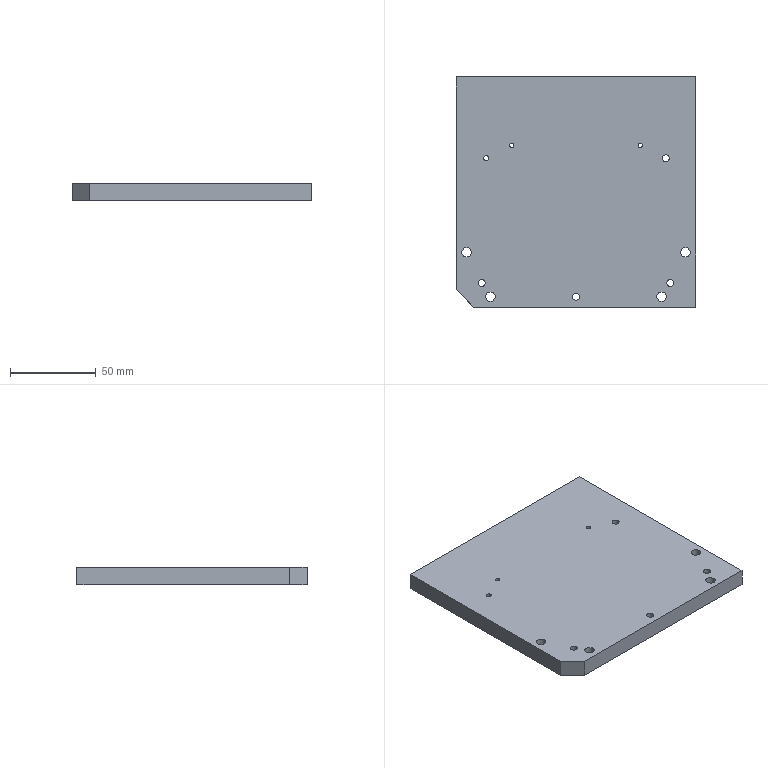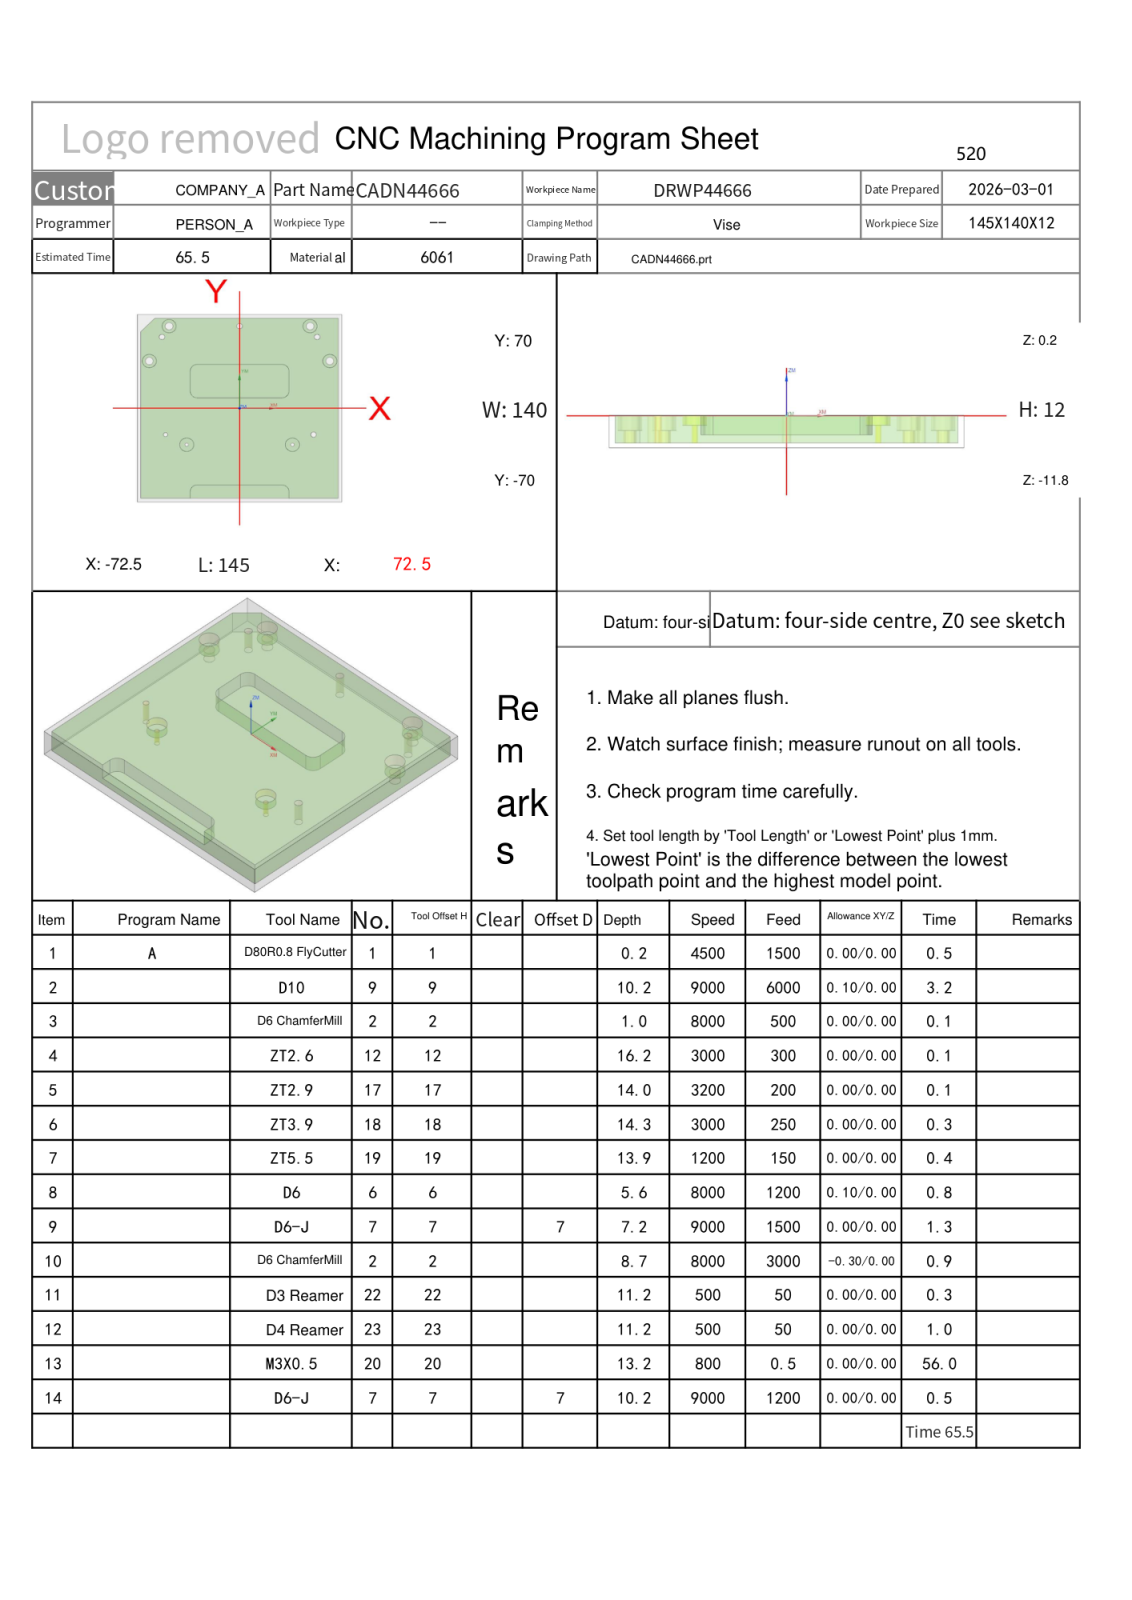NC program | NX | posted by the shop | part box 140 x 134.5 x 10 mm
Whole program:
%
O0001
(Machine time: 120.02 MIN)
(===Total Tool:12===)
(T1=D80R0.8 FlyCutter D=80.  R=0.8  D-  H01 Z=0.    )
(T9=D10     D=10.  R=0.   D9  H09 Z=-10.  )
(T2=D6 ChamferMill   D=6.   R=0.   D-  H02 Z=-8.5  )
(T12=ZT2.6  D=2.6  DR_a=118 D-  H12 Z=-16.  )
(T17=ZT2.9  D=2.9  DR_a=120 D-  H17 Z=-13.84)
(T18=ZT3.9  D=3.9  DR_a=120 D-  H18 Z=-14.13)
(T19=ZT5.5  D=5.5  DR_a=118 D-  H19 Z=-13.65)
(T6=D6      D=6.   R=0.   D-  H06 Z=-5.4  )
(T7=D6-J    D=6.   R=0.   D7  H07 Z=-10.  )
(T22=D3 Reamer   D=3.   DR_a=180 D-  H22 Z=-11.  )
(T23=D4 Reamer   D=4.   DR_a=180 D-  H23 Z=-11.  )
(T20=M3X0.5 D=2.5  DR_a=180 D-  H20 Z=-13.  )
G80 G90 G17 G49 G40
G91 G28 Z0
M01
N1 T01 M06
(D80R0.8 FlyCutter  D=80. R=0.8 H=01 ce=0.00 di=0.00)
G00 G90 G54 X115. Y-53.625 M03 S4500
G43 H01 Z50.
M08
Z2.
G01 Z0.0 F1500.
X110.
X-110.
Y0.0
X110.
Y53.625
X-110.
X-115.
Z2.
G00 Z50.
G91 G28 Z0.0
M05
M09
G91 G28 Z0.0
M01
N2 T09 M06
(D10  D=10. R=0. H=09 ce=0.10 di=0.00)
G00 G90 G54 X0.0 Y-72.35 M03 S8000
G43 H09 Z50.
M08
Z.5
G01 X-70. Z.409 F6000.
G02 X-75.1 Y-67.25 Z.398 I0.0 J5.1
G01 Y57.25 Z.236
G02 X-73.606 Y60.856 Z.231 I5.1 J0.0
G01 X-63.606 Y70.856 Z.212
G02 X-60. Y72.35 Z.207 I3.606 J-3.606
G01 X70. Z.038
G02 X75.1 Y67.25 Z.027 I0.0 J-5.1
G01 Y-67.25 Z-.148
G02 X70. Y-72.35 Z-.159 I-5.1 J0.0
G01 X-70. Z-.341
G02 X-75.1 Y-67.25 Z-.352 I0.0 J5.1
G01 Y57.25 Z-.514
G02 X-73.606 Y60.856 Z-.519 I5.1 J0.0
G01 X-63.606 Y70.856 Z-.538
G02 X-60. Y72.35 Z-.543 I3.606 J-3.606
G01 X70. Z-.712
G02 X75.1 Y67.25 Z-.723 I0.0 J-5.1
G01 Y-67.25 Z-.898
G02 X70. Y-72.35 Z-.909 I-5.1 J0.0
G01 X-70. Z-1.091
G02 X-75.1 Y-67.25 Z-1.102 I0.0 J5.1
G01 Y57.25 Z-1.264
G02 X-73.606 Y60.856 Z-1.269 I5.1 J0.0
G01 X-63.606 Y70.856 Z-1.288
G02 X-60. Y72.35 Z-1.293 I3.606 J-3.606
G01 X70. Z-1.462
G02 X75.1 Y67.25 Z-1.473 I0.0 J-5.1
G01 Y-67.25 Z-1.648
G02 X70. Y-72.35 Z-1.659 I-5.1 J0.0
G01 X-70. Z-1.841
G02 X-75.1 Y-67.25 Z-1.852 I0.0 J5.1
G01 Y57.25 Z-2.014
G02 X-73.606 Y60.856 Z-2.019 I5.1 J0.0
G01 X-63.606 Y70.856 Z-2.038
G02 X-60. Y72.35 Z-2.043 I3.606 J-3.606
G01 X70. Z-2.212
G02 X75.1 Y67.25 Z-2.223 I0.0 J-5.1
G01 Y-67.25 Z-2.398
G02 X70. Y-72.35 Z-2.409 I-5.1 J0.0
G01 X-70. Z-2.591
G02 X-75.1 Y-67.25 Z-2.602 I0.0 J5.1
G01 Y57.25 Z-2.764
G02 X-73.606 Y60.856 Z-2.769 I5.1 J0.0
G01 X-63.606 Y70.856 Z-2.788
G02 X-60. Y72.35 Z-2.793 I3.606 J-3.606
G01 X70. Z-2.962
G02 X75.1 Y67.25 Z-2.973 I0.0 J-5.1
G01 Y-67.25 Z-3.148
G02 X70. Y-72.35 Z-3.159 I-5.1 J0.0
G01 X-70. Z-3.341
G02 X-75.1 Y-67.25 Z-3.352 I0.0 J5.1
G01 Y57.25 Z-3.514
G02 X-73.606 Y60.856 Z-3.519 I5.1 J0.0
G01 X-63.606 Y70.856 Z-3.538
G02 X-60. Y72.35 Z-3.543 I3.606 J-3.606
G01 X70. Z-3.712
G02 X75.1 Y67.25 Z-3.723 I0.0 J-5.1
G01 Y-67.25 Z-3.898
G02 X70. Y-72.35 Z-3.909 I-5.1 J0.0
G01 X-70. Z-4.091
G02 X-75.1 Y-67.25 Z-4.102 I0.0 J5.1
G01 Y57.25 Z-4.264
G02 X-73.606 Y60.856 Z-4.269 I5.1 J0.0
G01 X-63.606 Y70.856 Z-4.288
G02 X-60. Y72.35 Z-4.293 I3.606 J-3.606
G01 X70. Z-4.462
G02 X75.1 Y67.25 Z-4.473 I0.0 J-5.1
G01 Y-67.25 Z-4.648
G02 X70. Y-72.35 Z-4.659 I-5.1 J0.0
G01 X-70. Z-4.841
G02 X-75.1 Y-67.25 Z-4.852 I0.0 J5.1
G01 Y57.25 Z-5.014
G02 X-73.606 Y60.856 Z-5.019 I5.1 J0.0
G01 X-63.606 Y70.856 Z-5.038
G02 X-60. Y72.35 Z-5.043 I3.606 J-3.606
G01 X70. Z-5.212
G02 X75.1 Y67.25 Z-5.223 I0.0 J-5.1
G01 Y-67.25 Z-5.398
G02 X70. Y-72.35 Z-5.409 I-5.1 J0.0
G01 X-70. Z-5.591
G02 X-75.1 Y-67.25 Z-5.602 I0.0 J5.1
G01 Y57.25 Z-5.764
G02 X-73.606 Y60.856 Z-5.769 I5.1 J0.0
G01 X-63.606 Y70.856 Z-5.788
G02 X-60. Y72.35 Z-5.793 I3.606 J-3.606
G01 X70. Z-5.962
G02 X75.1 Y67.25 Z-5.973 I0.0 J-5.1
G01 Y-67.25 Z-6.148
G02 X70. Y-72.35 Z-6.159 I-5.1 J0.0
G01 X-70. Z-6.341
G02 X-75.1 Y-67.25 Z-6.352 I0.0 J5.1
G01 Y57.25 Z-6.514
G02 X-73.606 Y60.856 Z-6.519 I5.1 J0.0
G01 X-63.606 Y70.856 Z-6.538
G02 X-60. Y72.35 Z-6.543 I3.606 J-3.606
G01 X70. Z-6.712
G02 X75.1 Y67.25 Z-6.723 I0.0 J-5.1
G01 Y-67.25 Z-6.898
G02 X70. Y-72.35 Z-6.909 I-5.1 J0.0
G01 X-70. Z-7.091
G02 X-75.1 Y-67.25 Z-7.102 I0.0 J5.1
G01 Y57.25 Z-7.264
G02 X-73.606 Y60.856 Z-7.269 I5.1 J0.0
G01 X-63.606 Y70.856 Z-7.288
G02 X-60. Y72.35 Z-7.293 I3.606 J-3.606
G01 X70. Z-7.462
G02 X75.1 Y67.25 Z-7.473 I0.0 J-5.1
G01 Y-67.25 Z-7.648
G02 X70. Y-72.35 Z-7.659 I-5.1 J0.0
G01 X-70. Z-7.841
G02 X-75.1 Y-67.25 Z-7.852 I0.0 J5.1
G01 Y57.25 Z-8.014
G02 X-73.606 Y60.856 Z-8.019 I5.1 J0.0
G01 X-63.606 Y70.856 Z-8.038
G02 X-60. Y72.35 Z-8.043 I3.606 J-3.606
G01 X70. Z-8.212
G02 X75.1 Y67.25 Z-8.223 I0.0 J-5.1
G01 Y-67.25 Z-8.398
G02 X70. Y-72.35 Z-8.409 I-5.1 J0.0
G01 X-70. Z-8.591
G02 X-75.1 Y-67.25 Z-8.602 I0.0 J5.1
G01 Y57.25 Z-8.764
G02 X-73.606 Y60.856 Z-8.769 I5.1 J0.0
G01 X-63.606 Y70.856 Z-8.788
G02 X-60. Y72.35 Z-8.793 I3.606 J-3.606
G01 X70. Z-8.962
G02 X75.1 Y67.25 Z-8.973 I0.0 J-5.1
G01 Y-67.25 Z-9.148
G02 X70. Y-72.35 Z-9.159 I-5.1 J0.0
G01 X-70. Z-9.341
G02 X-75.1 Y-67.25 Z-9.352 I0.0 J5.1
G01 Y57.25 Z-9.514
G02 X-73.606 Y60.856 Z-9.519 I5.1 J0.0
G01 X-63.606 Y70.856 Z-9.538
G02 X-60. Y72.35 Z-9.543 I3.606 J-3.606
G01 X70. Z-9.712
G02 X75.1 Y67.25 Z-9.723 I0.0 J-5.1
G01 Y-67.25 Z-9.898
G02 X70. Y-72.35 Z-9.909 I-5.1 J0.0
G01 X0.0 Z-10.
X-70.
G02 X-75.1 Y-67.25 I0.0 J5.1
G01 Y57.25
G02 X-73.606 Y60.856 I5.1 J0.0
G01 X-63.606 Y70.856
G02 X-60. Y72.35 I3.606 J-3.606
G01 X70.
G02 X75.1 Y67.25 I0.0 J-5.1
G01 Y-67.25
G02 X70. Y-72.35 I-5.1 J0.0
G01 X0.0
X-.5
Z-9.
G00 Z50.
G00 G90 X17.527 Y20.15 M03 S9000
Z50.
Z.7
M03 S9000
G01 X22.6 Z.523 F2800.
Y20.35 Z.516
X0.0 Z-.273
Y20.65
M03 S9000
X-22.9 F3500.
Y19.85
X22.9
Y20.65
X0.0
Y27.65
X-29.9
Y12.85
X29.9
Y27.65
X0.0
Z.727
G00 Z1.2
X17.527 Y20.15
Z.227
M03 S9000
G01 X22.6 Z.05 F2800.
Y20.35 Z.043
X0.0 Z-.747
Y20.65
M03 S9000
X-22.9 F3500.
Y19.85
X22.9
Y20.65
X0.0
Y27.65
X-29.9
Y12.85
X29.9
Y27.65
X0.0
Z.253
G00 Z.727
X17.527 Y20.15
Z-.247
M03 S9000
G01 X22.6 Z-.424 F2800.
Y20.35 Z-.431
X0.0 Z-1.22
Y20.65
M03 S9000
X-22.9 F3500.
Y19.85
X22.9
Y20.65
X0.0
Y27.65
X-29.9
Y12.85
X29.9
Y27.65
X0.0
Z-.22
G00 Z.253
X17.527 Y20.15
Z-.72
M03 S9000
G01 X22.6 Z-.897 F2800.
Y20.35 Z-.904
X0.0 Z-1.693
Y20.65
M03 S9000
X-22.9 F3500.
Y19.85
X22.9
Y20.65
X0.0
Y27.65
X-29.9
Y12.85
X29.9
Y27.65
X0.0
Z-.693
G00 Z-.22
X17.527 Y20.15
Z-1.193
M03 S9000
G01 X22.6 Z-1.37 F2800.
Y20.35 Z-1.377
X0.0 Z-2.167
Y20.65
M03 S9000
X-22.9 F3500.
Y19.85
X22.9
Y20.65
X0.0
Y27.65
X-29.9
Y12.85
X29.9
Y27.65
X0.0
Z-1.167
G00 Z-.693
X17.527 Y20.15
Z-1.667
M03 S9000
G01 X22.6 Z-1.844 F2800.
Y20.35 Z-1.851
X0.0 Z-2.64
Y20.65
M03 S9000
X-22.9 F3500.
Y19.85
X22.9
Y20.65
X0.0
Y27.65
X-29.9
Y12.85
X29.9
Y27.65
X0.0
Z-1.64
G00 Z-1.167
X17.527 Y20.15
Z-2.14
M03 S9000
G01 X22.6 Z-2.317 F2800.
Y20.35 Z-2.324
X0.0 Z-3.113
Y20.65
M03 S9000
X-22.9 F3500.
Y19.85
X22.9
Y20.65
X0.0
Y27.65
X-29.9
Y12.85
X29.9
Y27.65
X0.0
Z-2.113
G00 Z-1.64
X17.527 Y20.15
Z-2.613
M03 S9000
G01 X22.6 Z-2.79 F2800.
Y20.35 Z-2.797
X0.0 Z-3.587
Y20.65
M03 S9000
X-22.9 F3500.
Y19.85
X22.9
Y20.65
X0.0
Y27.65
X-29.9
Y12.85
X29.9
Y27.65
X0.0
Z-2.587
G00 Z-2.113
X17.527 Y20.15
Z-3.087
M03 S9000
G01 X22.6 Z-3.264 F2800.
Y20.35 Z-3.271
X0.0 Z-4.06
Y20.65
M03 S9000
X-22.9 F3500.
Y19.85
X22.9
Y20.65
X0.0
Y27.65
X-29.9
Y12.85
X29.9
Y27.65
X0.0
Z-3.06
G00 Z-2.587
X17.527 Y20.15
Z-3.56
M03 S9000
G01 X22.6 Z-3.737 F2800.
Y20.35 Z-3.744
X0.0 Z-4.533
Y20.65
M03 S9000
X-22.9 F3500.
Y19.85
X22.9
Y20.65
X0.0
Y27.65
X-29.9
Y12.85
X29.9
Y27.65
X0.0
Z-3.533
G00 Z-3.06
X17.527 Y20.15
Z-4.033
M03 S9000
G01 X22.6 Z-4.21 F2800.
Y20.35 Z-4.217
X0.0 Z-5.007
Y20.65
M03 S9000
X-22.9 F3500.
Y19.85
X22.9
Y20.65
X0.0
Y27.65
X-29.9
Y12.85
X29.9
Y27.65
X0.0
Z-4.007
G00 Z-3.533
X17.527 Y20.15
Z-4.507
M03 S9000
G01 X22.6 Z-4.684 F2800.
Y20.35 Z-4.691
X0.0 Z-5.48
Y20.65
M03 S9000
X-22.9 F3500.
Y19.85
X22.9
Y20.65
X0.0
Y27.65
X-29.9
Y12.85
X29.9
Y27.65
X0.0
Z-4.48
G00 Z-4.007
X17.527 Y20.15
Z-4.98
M03 S9000
G01 X22.6 Z-5.157 F2800.
Y20.35 Z-5.164
X0.0 Z-5.953
Y20.65
M03 S9000
X-22.9 F3500.
Y19.85
X22.9
Y20.65
X0.0
Y27.65
X-29.9
Y12.85
X29.9
Y27.65
X0.0
Z-4.953
G00 Z-4.48
X17.527 Y20.15
Z-5.453
M03 S9000
G01 X22.6 Z-5.63 F2800.
Y20.35 Z-5.637
X0.0 Z-6.427
Y20.65
M03 S9000
X-22.9 F3500.
Y19.85
X22.9
Y20.65
X0.0
Y27.65
X-29.9
Y12.85
X29.9
Y27.65
X0.0
Z-5.427
G00 Z-4.953
X17.527 Y20.15
Z-5.927
M03 S9000
G01 X22.6 Z-6.104 F2800.
Y20.35 Z-6.111
X0.0 Z-6.9
Y20.65
M03 S9000
X-22.9 F3500.
Y19.85
X22.9
Y20.65
X0.0
Y27.65
X-29.9
Y12.85
X29.9
Y27.65
X0.0
Z-5.9
G00 Z50.
G00 G90 X28.8 Y-72.75 M03 S9000
Z50.
Z.007
G01 Z-.493 F5000.
G41 D09
X28.9
G03 X29.9 Y-71.75 I0.0 J1.
G01 Y-62.35
X-29.9
Y-71.75
G03 X-28.9 Y-72.75 I1. J0.0
G01 G40 X-28.8
Z.007
G00 Z50.
X28.8
Z-.486
G01 Z-.986
G41 D09
X28.9
G03 X29.9 Y-71.75 I0.0 J1.
G01 Y-62.35
X-29.9
Y-71.75
G03 X-28.9 Y-72.75 I1. J0.0
G01 G40 X-28.8
Z-.486
G00 Z50.
X28.8
Z-.979
G01 Z-1.479
G41 D09
X28.9
G03 X29.9 Y-71.75 I0.0 J1.
G01 Y-62.35
X-29.9
Y-71.75
G03 X-28.9 Y-72.75 I1. J0.0
G01 G40 X-28.8
Z-.979
G00 Z50.
X28.8
Z-1.471
G01 Z-1.971
G41 D09
X28.9
G03 X29.9 Y-71.75 I0.0 J1.
G01 Y-62.35
X-29.9
Y-71.75
G03 X-28.9 Y-72.75 I1. J0.0
G01 G40 X-28.8
Z-1.471
G00 Z50.
X28.8
Z-1.964
G01 Z-2.464
G41 D09
X28.9
G03 X29.9 Y-71.75 I0.0 J1.
G01 Y-62.35
X-29.9
Y-71.75
G03 X-28.9 Y-72.75 I1. J0.0
G01 G40 X-28.8
Z-1.964
G00 Z50.
X28.8
Z-2.457
G01 Z-2.957
G41 D09
X28.9
G03 X29.9 Y-71.75 I0.0 J1.
G01 Y-62.35
X-29.9
Y-71.75
G03 X-28.9 Y-72.75 I1. J0.0
G01 G40 X-28.8
Z-2.457
G00 Z50.
X28.8
Z-2.95
G01 Z-3.45
G41 D09
X28.9
G03 X29.9 Y-71.75 I0.0 J1.
G01 Y-62.35
X-29.9
Y-71.75
G03 X-28.9 Y-72.75 I1. J0.0
G01 G40 X-28.8
Z-2.95
G00 Z50.
X28.8
Z-3.443
G01 Z-3.943
G41 D09
X28.9
G03 X29.9 Y-71.75 I0.0 J1.
G01 Y-62.35
X-29.9
Y-71.75
G03 X-28.9 Y-72.75 I1. J0.0
G01 G40 X-28.8
Z-3.443
G00 Z50.
X28.8
Z-3.936
G01 Z-4.436
G41 D09
X28.9
G03 X29.9 Y-71.75 I0.0 J1.
G01 Y-62.35
X-29.9
Y-71.75
G03 X-28.9 Y-72.75 I1. J0.0
G01 G40 X-28.8
Z-3.936
G00 Z50.
X28.8
Z-4.429
G01 Z-4.929
G41 D09
X28.9
G03 X29.9 Y-71.75 I0.0 J1.
G01 Y-62.35
X-29.9
Y-71.75
G03 X-28.9 Y-72.75 I1. J0.0
G01 G40 X-28.8
Z-4.429
G00 Z50.
X28.8
Z-4.921
G01 Z-5.421
G41 D09
X28.9
G03 X29.9 Y-71.75 I0.0 J1.
G01 Y-62.35
X-29.9
Y-71.75
G03 X-28.9 Y-72.75 I1. J0.0
G01 G40 X-28.8
Z-4.921
G00 Z50.
X28.8
Z-5.414
G01 Z-5.914
G41 D09
X28.9
G03 X29.9 Y-71.75 I0.0 J1.
G01 Y-62.35
X-29.9
Y-71.75
G03 X-28.9 Y-72.75 I1. J0.0
G01 G40 X-28.8
Z-5.414
G00 Z50.
X28.8
Z-5.907
G01 Z-6.407
G41 D09
X28.9
G03 X29.9 Y-71.75 I0.0 J1.
G01 Y-62.35
X-29.9
Y-71.75
G03 X-28.9 Y-72.75 I1. J0.0
G01 G40 X-28.8
Z-5.907
G00 Z50.
X28.8
Z-6.4
G01 Z-6.9
G41 D09
X28.9
G03 X29.9 Y-71.75 I0.0 J1.
G01 Y-62.35
X-29.9
Y-71.75
G03 X-28.9 Y-72.75 I1. J0.0
G01 G40 X-28.8
Z-6.4
G00 Z50.
G91 G28 Z0.0
M05
M09
G91 G28 Z0.0
M01
N3 T02 M06
(D6 ChamferMill  D=6. R=0. H=02 ce=0.00 di=0.10)
G00 G90 G54 X37.5 Y-27.25 M03 S8000
G43 H02 Z50.
M08
G98 G81 X37.5 Y-27.25 Z-.8 R1. F500.
X52.5 Y-19.75
X64. Y35.25
X55. Y53.25
X50. Y61.25
X0.0
X-50.
X-55. Y53.25
X-64. Y35.25
X-52.5 Y-19.75
X-37.5 Y-27.25
G80
G00 Z50.
G00 G90 X37.5 Y-27.25 M03 S8000
Z50.
G98 G81 X37.5 Y-27.25 Z-.8 R1. F500.
X-37.5
G80
G00 Z50.
G91 G28 Z0.0
M05
M09
G91 G28 Z0.0
M01
N4 T12 M06
(ZT2.6 D=2.6 DR_a=118 H=12)
G00 G90 G54 X37.5 Y-27.25 M03 S3000
G43 H12 Z50.
M08
G98 G83 X37.5 Y-27.25 Z-16. R1. F300. Q2.
X-37.5
G80
G00 Z50.
G91 G28 Z0.0
M05
M09
G91 G28 Z0.0
M01
N5 T17 M06
(ZT2.9 D=2.9 DR_a=120 H=17)
G00 G90 G54 X-52.5 Y-19.75 M03 S3200
G43 H17 Z50.
M08
G98 G83 X-52.5 Y-19.75 Z-13.837 R1. F200. Q2.
G80
G00 Z50.
G91 G28 Z0.0
M05
M09
G91 G28 Z0.0
M01
N6 T18 M06
(ZT3.9 D=3.9 DR_a=120 H=18)
G00 G90 G54 X-55. Y53.25 M03 S3000
G43 H18 Z50.
M08
G98 G83 X-55. Y53.25 Z-14.126 R1. F250. Q2.
X0.0 Y61.25
X55. Y53.25
X52.5 Y-19.75
G80
G00 Z50.
G91 G28 Z0.0
M05
M09
G91 G28 Z0.0
M01
N7 T19 M06
(ZT5.5 D=5.5 DR_a=118 H=19)
G00 G90 G54 X-64. Y35.25 M03 S1200
G43 H19 Z50.
M08
G98 G83 X-64. Y35.25 Z-13.652 R1. F150. Q2.
X-50. Y61.25
X50.
X64. Y35.25
G80
G00 Z50.
G91 G28 Z0.0
M05
M09
G91 G28 Z0.0
M01
N8 T06 M06
(D6  D=6. R=0. H=06 ce=0.10 di=0.00)
G00 G90 G54 X-64. Y35.25 M03 S8000
G43 H06 Z50.
M08
Z.5
G03 X-63.05 Y34.3 I.95 J0.0 F1200.
X-62.1 Y35.25 I0.0 J.95
X-62.1 Y35.25 Z0.0 I-1.9 J0.0
X-62.1 Y35.25 Z-.5 I-1.9 J0.0
X-62.1 Y35.25 Z-1. I-1.9 J0.0
X-62.1 Y35.25 Z-1.5 I-1.9 J0.0
X-62.1 Y35.25 Z-2. I-1.9 J0.0
X-62.1 Y35.25 Z-2.5 I-1.9 J0.0
X-62.1 Y35.25 Z-3. I-1.9 J0.0
X-62.1 Y35.25 Z-3.5 I-1.9 J0.0
X-62.1 Y35.25 Z-4. I-1.9 J0.0
X-62.1 Y35.25 Z-4.5 I-1.9 J0.0
X-62.1 Y35.25 Z-5. I-1.9 J0.0
X-63.413 Y33.443 Z-5.4 I-1.9 J0.0
X-62.1 Y35.25 I-.587 J1.807
X-64. Y37.15 I-1.9 J0.0
X-65.9 Y35.25 I0.0 J-1.9
X-64. Y33.35 I1.9 J0.0
X-63.413 Y33.443 I0.0 J1.9
X-62.756 Y34.346 I-.294 J.904
X-63.706 Y35.296 I-.95 J0.0
X-64. Y35.25 I0.0 J-.95
G00 Z50.
X-50. Y61.25
Z.5
G03 X-49.05 Y60.3 I.95 J0.0
X-48.1 Y61.25 I0.0 J.95
X-48.1 Y61.25 Z0.0 I-1.9 J0.0
X-48.1 Y61.25 Z-.5 I-1.9 J0.0
X-48.1 Y61.25 Z-1. I-1.9 J0.0
X-48.1 Y61.25 Z-1.5 I-1.9 J0.0
X-48.1 Y61.25 Z-2. I-1.9 J0.0
X-48.1 Y61.25 Z-2.5 I-1.9 J0.0
X-48.1 Y61.25 Z-3. I-1.9 J0.0
X-48.1 Y61.25 Z-3.5 I-1.9 J0.0
X-48.1 Y61.25 Z-4. I-1.9 J0.0
X-48.1 Y61.25 Z-4.5 I-1.9 J0.0
X-48.1 Y61.25 Z-5. I-1.9 J0.0
X-49.413 Y59.443 Z-5.4 I-1.9 J0.0
X-48.1 Y61.25 I-.587 J1.807
X-50. Y63.15 I-1.9 J0.0
X-51.9 Y61.25 I0.0 J-1.9
X-50. Y59.35 I1.9 J0.0
X-49.413 Y59.443 I0.0 J1.9
X-48.756 Y60.346 I-.294 J.904
X-49.706 Y61.296 I-.95 J0.0
X-50. Y61.25 I0.0 J-.95
G00 Z50.
X50.
Z.5
G03 X50.95 Y60.3 I.95 J0.0
X51.9 Y61.25 I0.0 J.95
X51.9 Y61.25 Z0.0 I-1.9 J0.0
X51.9 Y61.25 Z-.5 I-1.9 J0.0
X51.9 Y61.25 Z-1. I-1.9 J0.0
X51.9 Y61.25 Z-1.5 I-1.9 J0.0
X51.9 Y61.25 Z-2. I-1.9 J0.0
X51.9 Y61.25 Z-2.5 I-1.9 J0.0
X51.9 Y61.25 Z-3. I-1.9 J0.0
X51.9 Y61.25 Z-3.5 I-1.9 J0.0
X51.9 Y61.25 Z-4. I-1.9 J0.0
X51.9 Y61.25 Z-4.5 I-1.9 J0.0
X51.9 Y61.25 Z-5. I-1.9 J0.0
X50.587 Y59.443 Z-5.4 I-1.9 J0.0
X51.9 Y61.25 I-.587 J1.807
X50. Y63.15 I-1.9 J0.0
X48.1 Y61.25 I0.0 J-1.9
X50. Y59.35 I1.9 J0.0
X50.587 Y59.443 I0.0 J1.9
X51.244 Y60.346 I-.294 J.904
X50.294 Y61.296 I-.95 J0.0
X50. Y61.25 I0.0 J-.95
G00 Z50.
X64. Y35.25
Z.5
G03 X64.95 Y34.3 I.95 J0.0
X65.9 Y35.25 I0.0 J.95
X65.9 Y35.25 Z0.0 I-1.9 J0.0
X65.9 Y35.25 Z-.5 I-1.9 J0.0
X65.9 Y35.25 Z-1. I-1.9 J0.0
X65.9 Y35.25 Z-1.5 I-1.9 J0.0
X65.9 Y35.25 Z-2. I-1.9 J0.0
X65.9 Y35.25 Z-2.5 I-1.9 J0.0
X65.9 Y35.25 Z-3. I-1.9 J0.0
X65.9 Y35.25 Z-3.5 I-1.9 J0.0
X65.9 Y35.25 Z-4. I-1.9 J0.0
X65.9 Y35.25 Z-4.5 I-1.9 J0.0
X65.9 Y35.25 Z-5. I-1.9 J0.0
X64.587 Y33.443 Z-5.4 I-1.9 J0.0
X65.9 Y35.25 I-.587 J1.807
X64. Y37.15 I-1.9 J0.0
X62.1 Y35.25 I0.0 J-1.9
X64. Y33.35 I1.9 J0.0
X64.587 Y33.443 I0.0 J1.9
X65.244 Y34.346 I-.294 J.904
X64.294 Y35.296 I-.95 J0.0
X64. Y35.25 I0.0 J-.95
G00 Z50.
G00 G90 X-37.5 Y-27.25 M03 S8000
Z50.
Z.5
G03 X-36.525 Y-28.225 I.975 J0.0 F1200.
X-35.55 Y-27.25 I0.0 J.975
X-35.55 Y-27.25 Z0.0 I-1.95 J0.0
X-35.55 Y-27.25 Z-.5 I-1.95 J0.0
X-35.55 Y-27.25 Z-1. I-1.95 J0.0
X-35.55 Y-27.25 Z-1.5 I-1.95 J0.0
X-35.55 Y-27.25 Z-2. I-1.95 J0.0
X-35.55 Y-27.25 Z-2.5 I-1.95 J0.0
X-35.55 Y-27.25 Z-3. I-1.95 J0.0
X-35.55 Y-27.25 Z-3.5 I-1.95 J0.0
X-37.5 Y-25.3 I-1.95 J0.0
X-39.45 Y-27.25 I0.0 J-1.95
X-37.5 Y-29.2 I1.95 J0.0
X-35.55 Y-27.25 I0.0 J1.95
X-36.525 Y-26.275 I-.975 J0.0
X-37.5 Y-27.25 I0.0 J-.975
G00 Z50.
X37.5
Z.5
G03 X38.475 Y-28.225 I.975 J0.0
X39.45 Y-27.25 I0.0 J.975
X39.45 Y-27.25 Z0.0 I-1.95 J0.0
X39.45 Y-27.25 Z-.5 I-1.95 J0.0
X39.45 Y-27.25 Z-1. I-1.95 J0.0
X39.45 Y-27.25 Z-1.5 I-1.95 J0.0
X39.45 Y-27.25 Z-2. I-1.95 J0.0
X39.45 Y-27.25 Z-2.5 I-1.95 J0.0
X39.45 Y-27.25 Z-3. I-1.95 J0.0
X39.45 Y-27.25 Z-3.5 I-1.95 J0.0
X37.5 Y-25.3 I-1.95 J0.0
X35.55 Y-27.25 I0.0 J-1.95
X37.5 Y-29.2 I1.95 J0.0
X39.45 Y-27.25 I0.0 J1.95
X38.475 Y-26.275 I-.975 J0.0
X37.5 Y-27.25 I0.0 J-.975
G00 Z50.
G91 G28 Z0.0
M05
M09
G91 G28 Z0.0
M01
N9 T07 M06
(D6-J  D=6. R=0. H=07 ce=0.00 di=0.00)
G00 G90 G54 X-64. Y35.25 M03 S8000
G43 H07 Z50.
M08
Z0.0
G41 D07
G01 X-63.96 Y35.054 F500.
G03 X-62.99 Y34.26 I.97 J.196
X-62. Y35.25 I0.0 J.99
X-62. Y35.25 Z-5. I-2. J0.0
X-62.247 Y36.214 Z-5.4 I-2. J0.0
X-64. Y37.25 I-1.753 J-.964
X-66. Y35.25 I0.0 J-2.
X-64. Y33.25 I2. J0.0
X-62. Y35.25 I0.0 J2.
X-62.247 Y36.214 I-2. J0.0
X-63.115 Y36.727 I-.868 J-.477
X-64.105 Y35.737 I0.0 J-.99
X-64.06 Y35.441 I.99 J0.0
G01 G40 X-64. Y35.25
G00 Z50.
X-50. Y61.25
Z0.0
G41 D07
G01 X-49.96 Y61.054
G03 X-48.99 Y60.26 I.97 J.196
X-48. Y61.25 I0.0 J.99
X-48. Y61.25 Z-5. I-2. J0.0
X-48.247 Y62.214 Z-5.4 I-2. J0.0
X-50. Y63.25 I-1.753 J-.964
X-52. Y61.25 I0.0 J-2.
X-50. Y59.25 I2. J0.0
X-48. Y61.25 I0.0 J2.
X-48.247 Y62.214 I-2. J0.0
X-49.115 Y62.727 I-.868 J-.477
X-50.105 Y61.737 I0.0 J-.99
X-50.06 Y61.441 I.99 J0.0
G01 G40 X-50. Y61.25
G00 Z50.
X50.
Z0.0
G41 D07
G01 X50.04 Y61.054
G03 X51.01 Y60.26 I.97 J.196
X52. Y61.25 I0.0 J.99
X52. Y61.25 Z-5. I-2. J0.0
X51.753 Y62.214 Z-5.4 I-2. J0.0
X50. Y63.25 I-1.753 J-.964
X48. Y61.25 I0.0 J-2.
X50. Y59.25 I2. J0.0
X52. Y61.25 I0.0 J2.
X51.753 Y62.214 I-2. J0.0
X50.885 Y62.727 I-.868 J-.477
X49.895 Y61.737 I0.0 J-.99
X49.94 Y61.441 I.99 J0.0
G01 G40 X50. Y61.25
G00 Z50.
X64. Y35.25
Z0.0
G41 D07
G01 X64.04 Y35.054
G03 X65.01 Y34.26 I.97 J.196
X66. Y35.25 I0.0 J.99
X66. Y35.25 Z-5. I-2. J0.0
X65.753 Y36.214 Z-5.4 I-2. J0.0
X64. Y37.25 I-1.753 J-.964
X62. Y35.25 I0.0 J-2.
X64. Y33.25 I2. J0.0
X66. Y35.25 I0.0 J2.
X65.753 Y36.214 I-2. J0.0
X64.885 Y36.727 I-.868 J-.477
X63.895 Y35.737 I0.0 J-.99
X63.94 Y35.441 I.99 J0.0
G01 G40 X64. Y35.25
G00 Z50.
G00 G90 X-37.5 Y-27.25 M03 S8000
Z50.
Z0.0
G41 D07
G01 X-37.461 Y-27.446 F500.
G03 X-36.465 Y-28.265 I.996 J.196
X-35.45 Y-27.25 I0.0 J1.015
X-38.133 Y-29.2 Z-3.5 I-2.05 J0.0
X-37.5 Y-29.3 I.633 J1.95
X-35.45 Y-27.25 I0.0 J2.05
X-37.5 Y-25.2 I-2.05 J0.0
X-39.55 Y-27.25 I0.0 J-2.05
X-38.133 Y-29.2 I2.05 J0.0
X-37.82 Y-29.249 I.314 J.966
X-36.805 Y-28.234 I0.0 J1.015
X-37.325 Y-27.347 I-1.015 J0.0
G01 G40 X-37.5 Y-27.25
G00 Z50.
X37.5
Z0.0
G41 D07
G01 X37.539 Y-27.446
G03 X38.535 Y-28.265 I.996 J.196
X39.55 Y-27.25 I0.0 J1.015
X36.867 Y-29.2 Z-3.5 I-2.05 J0.0
X37.5 Y-29.3 I.633 J1.95
X39.55 Y-27.25 I0.0 J2.05
X37.5 Y-25.2 I-2.05 J0.0
X35.45 Y-27.25 I0.0 J-2.05
X36.867 Y-29.2 I2.05 J0.0
X37.18 Y-29.249 I.314 J.966
X38.195 Y-28.234 I0.0 J1.015
X37.675 Y-27.347 I-1.015 J0.0
G01 G40 X37.5 Y-27.25
G00 Z50.
G00 G90 X-31.7 Y17.474 M03 S8000
Z50.
Z-5.5
G01 Y27.935 Z-5.865 F1200.
X-31.589 Y28.383 Z-5.881
X-31.361 Y28.785 Z-5.898
X-31.035 Y29.111 Z-5.914
X-30.633 Y29.339 Z-5.93
X-30.185 Y29.45 Z-5.946
X0.0 Z-7.
X30.
G02 X31.7 Y27.75 I0.0 J-1.7
G01 Y12.75
G02 X30. Y11.05 I-1.7 J0.0
G01 X-30.
G02 X-31.7 Y12.75 I0.0 J1.7
G01 Y27.75
G02 X-30. Y29.45 I1.7 J0.0
G01 X0.0
Y25.25
X27.5
Y15.25
X-27.5
Y25.25
X0.0
Y21.05
X23.3
Y19.45
X-23.3
Y21.05
X0.0
X.5
Y24.65
Z-6.5
G00 Z50.
G00 G90 X1.2 Y-71.45 M03 S7000
Z10.4
Z-5.5
G01 Z-7. F1500.
Y-69.05
G03 X0.0 Y-67.85 I-1.2 J0.0
G01 X-31.002
G02 X-31.6 Y-67.252 I.002 J.6
G01 Y-62.25
G02 X-30. Y-60.65 I1.6 J0.0
G01 X30.
G02 X31.6 Y-62.25 I0.0 J-1.6
G01 Y-67.252
G02 X31.002 Y-67.85 I-.6 J.002
G01 X-1.252
G02 X-1.675 Y-67.675 I0.0 J.6
G01 X-4.325 Y-65.025
G03 X-4.748 Y-64.85 I-.424 J-.425
G01 X-28.002
G02 X-28.6 Y-64.25 I.002 J.6
X-28.002 Y-63.65 I.6 J0.0
G01 X28.002
G02 X28.6 Y-64.25 I-.002 J-.6
X28.002 Y-64.85 I-.6 J0.0
G01 X-3.
X-4.
G03 X-5.2 Y-66.05 I0.0 J-1.2
G01 Y-71.45
Z-5.5
G00 Z10.4
G00 G90 X1. Y28.65 M03 S8000
Z50.
Z-6.495
G01 Z-6.995 F1200.
G41 D07
Y28.75
G03 X0.0 Y29.75 I-1. J0.0
G01 X-30.
G03 X-32. Y27.75 I0.0 J-2.
G01 Y12.75
G03 X-30. Y10.75 I2. J0.0
G01 X30.
G03 X32. Y12.75 I0.0 J2.
G01 Y27.75
G03 X30. Y29.75 I-2. J0.0
G01 X0.0
X-.5
G03 X-1.5 Y28.75 I0.0 J-1.
G01 G40 Y28.65
Z-6.495
G00 Z50.
G00 G90 X30.9 Y-70.95 M03 S9000
Z50.
Z-6.5
G01 Z-7. F1500.
G41 D07
X31.
G03 X32. Y-69.95 I0.0 J1.
G01 Y-62.25
G03 X30. Y-60.25 I-2. J0.0
G01 X-30.
G03 X-32. Y-62.25 I0.0 J-2.
G01 Y-69.95
G03 X-31. Y-70.95 I1. J0.0
G01 G40 X-30.9
Z-6.5
G00 Z50.
G91 G28 Z0.0
M05
M09
G91 G28 Z0.0
M01
N10 T02 M06
(D6 ChamferMill  D=6. R=0. H=02 ce=0.00 di=0.00)
G00 G90 G54 X72.128 Y.25 M03 S8000
G43 H02 Z50.
M08
Z2.099
G01 Z-1.5 F3000.
G03 X71.828 Y.33 I-.3 J-.52
X71.308 Y.03 I0.0 J-.6
G01 X71.3 Y0.0
Y-67.25
G02 X70. Y-68.55 I-1.3 J0.0
G01 X35.
G02 X33.7 Y-67.25 I0.0 J1.3
G01 Y-62.25
G03 X30. Y-58.55 I-3.7 J0.0
G01 X-30.
G03 X-33.7 Y-62.25 I0.0 J-3.7
G01 Y-67.25
G02 X-35. Y-68.55 I-1.3 J0.0
G01 X-70.
G02 X-71.3 Y-67.25 I0.0 J1.3
G01 Y57.25
X-71.275 Y57.504
X-71.201 Y57.747
X-71.081 Y57.972
X-70.919 Y58.169
X-60.919 Y68.169
X-60.722 Y68.331
X-60.497 Y68.451
X-60.254 Y68.525
X-60. Y68.55
X70.
G02 X71.3 Y67.25 I0.0 J-1.3
G01 Y0.0
X71.308 Y-.03
G03 X71.828 Y-.33 I.52 J.3
X72.128 Y-.25 I0.0 J.6
G01 Z2.099
G00 Z50.
X-.25 Y9.878
Z2.099
G01 Z-1.5
G03 X-.33 Y9.578 I.52 J-.3
X-.03 Y9.058 I.6 J0.0
G01 X0.0 Y9.05
X30.
G03 X33.7 Y12.75 I0.0 J3.7
G01 Y27.75
G03 X30. Y31.45 I-3.7 J0.0
G01 X-30.
G03 X-33.7 Y27.75 I0.0 J-3.7
G01 Y12.75
G03 X-30. Y9.05 I3.7 J0.0
G01 X0.0
X.03 Y9.058
G03 X.33 Y9.578 I-.3 J.52
X.25 Y9.878 I-.6 J0.0
G01 Z2.099
G00 Z50.
X31.968 Y-69.378
Z1.755
G01 Z-8.499
G03 X32.049 Y-69.078 I-.52 J.3
X31.749 Y-68.558 I-.6 J0.0
G01 X31.719 Y-68.55
X-31.719
X-31.749 Y-68.558
G03 X-32.049 Y-69.078 I.3 J-.52
X-31.968 Y-69.378 I.6 J0.0
G01 Z1.755
G00 Z50.
G00 G90 X-52.5 Y-19.75 M03 S8000
Z50.
G98 G81 X-52.5 Y-19.75 Z-1.8 R3. F500.
G80
G00 Z50.
G00 G90 X-55. Y53.25 M03 S8000
Z50.
G98 G81 X-55. Y53.25 Z-2.3 R3. F500.
X0.0 Y61.25
X55. Y53.25
X52.5 Y-19.75
G80
G00 Z50.
G00 G90 X66.654 Y38.636 M03 S8000
Z50.
Z2.5
G01 X66.645 Y38.644 Z2.495 F800.
X66.289 Y38.894 Z2.337
X66.011 Y39.054 Z2.22
X65.617 Y39.238 Z2.062
X65.207 Y39.38 Z1.904
X64.784 Y39.481 Z1.746
X64.354 Y39.538 Z1.588
X63.92 Y39.552 Z1.43
X63.486 Y39.522 Z1.272
X63.058 Y39.449 Z1.114
X62.64 Y39.332 Z.956
X62.235 Y39.174 Z.797
X61.849 Y38.977 Z.639
X61.484 Y38.741 Z.481
X61.145 Y38.469 Z.323
X60.835 Y38.165 Z.165
X60.557 Y37.831 Z.007
X60.314 Y37.471 Z-.151
X60.109 Y37.088 Z-.309
X59.944 Y36.686 Z-.467
X59.82 Y36.27 Z-.625
X59.738 Y35.843 Z-.783
X59.7 Y35.411 Z-.942
Y35.25 Z-1.
G03 X64. Y30.95 I4.3 J0.0
X68.3 Y35.25 I0.0 J4.3
X64. Y39.55 I-4.3 J0.0
X59.7 Y35.25 I0.0 J-4.3
X59.729 Y34.751 I4.3 J0.0
G01 Z1.5
G00 Z50.
X52.654 Y64.636
Z2.5
G01 X52.645 Y64.644 Z2.495
X52.289 Y64.894 Z2.337
X52.011 Y65.054 Z2.22
X51.617 Y65.238 Z2.062
X51.207 Y65.38 Z1.904
X50.784 Y65.481 Z1.746
X50.354 Y65.538 Z1.588
X49.92 Y65.552 Z1.43
X49.486 Y65.522 Z1.272
X49.058 Y65.449 Z1.114
X48.64 Y65.332 Z.956
X48.235 Y65.174 Z.797
X47.849 Y64.977 Z.639
X47.484 Y64.741 Z.481
X47.145 Y64.469 Z.323
X46.835 Y64.165 Z.165
X46.557 Y63.831 Z.007
X46.314 Y63.471 Z-.151
X46.109 Y63.088 Z-.309
X45.944 Y62.686 Z-.467
X45.82 Y62.27 Z-.625
X45.738 Y61.843 Z-.783
X45.7 Y61.411 Z-.942
Y61.25 Z-1.
G03 X50. Y56.95 I4.3 J0.0
X54.3 Y61.25 I0.0 J4.3
X50. Y65.55 I-4.3 J0.0
X45.7 Y61.25 I0.0 J-4.3
X45.729 Y60.751 I4.3 J0.0
G01 Z1.5
G00 Z50.
X-47.346 Y64.636
Z2.5
G01 X-47.355 Y64.644 Z2.495
X-47.711 Y64.894 Z2.337
X-47.989 Y65.054 Z2.22
X-48.383 Y65.238 Z2.062
X-48.793 Y65.38 Z1.904
X-49.216 Y65.481 Z1.746
X-49.646 Y65.538 Z1.588
X-50.08 Y65.552 Z1.43
X-50.514 Y65.522 Z1.272
X-50.942 Y65.449 Z1.114
X-51.36 Y65.332 Z.956
X-51.765 Y65.174 Z.797
X-52.152 Y64.977 Z.639
X-52.516 Y64.741 Z.481
X-52.855 Y64.469 Z.323
X-53.165 Y64.165 Z.165
X-53.443 Y63.831 Z.007
X-53.686 Y63.471 Z-.151
X-53.891 Y63.088 Z-.309
X-54.056 Y62.686 Z-.467
X-54.18 Y62.27 Z-.625
X-54.262 Y61.843 Z-.783
X-54.3 Y61.411 Z-.942
Y61.25 Z-1.
G03 X-50. Y56.95 I4.3 J0.0
X-45.7 Y61.25 I0.0 J4.3
X-50. Y65.55 I-4.3 J0.0
X-54.3 Y61.25 I0.0 J-4.3
X-54.271 Y60.751 I4.3 J0.0
G01 Z1.5
G00 Z50.
X-61.346 Y38.636
Z2.5
G01 X-61.355 Y38.644 Z2.495
X-61.711 Y38.894 Z2.337
X-61.989 Y39.054 Z2.22
X-62.383 Y39.238 Z2.062
X-62.793 Y39.38 Z1.904
X-63.216 Y39.481 Z1.746
X-63.646 Y39.538 Z1.588
X-64.08 Y39.552 Z1.43
X-64.514 Y39.522 Z1.272
X-64.942 Y39.449 Z1.114
X-65.36 Y39.332 Z.956
X-65.765 Y39.174 Z.797
X-66.152 Y38.977 Z.639
X-66.516 Y38.741 Z.481
X-66.855 Y38.469 Z.323
X-67.165 Y38.165 Z.165
X-67.443 Y37.831 Z.007
X-67.686 Y37.471 Z-.151
X-67.891 Y37.088 Z-.309
X-68.056 Y36.686 Z-.467
X-68.18 Y36.27 Z-.625
X-68.262 Y35.843 Z-.783
X-68.3 Y35.411 Z-.942
Y35.25 Z-1.
G03 X-64. Y30.95 I4.3 J0.0
X-59.7 Y35.25 I0.0 J4.3
X-64. Y39.55 I-4.3 J0.0
X-68.3 Y35.25 I0.0 J-4.3
X-68.271 Y34.751 I4.3 J0.0
G01 Z1.5
G00 Z50.
G00 G90 X-34.905 Y-23.76 M03 S8000
Z50.
Z2.5
G01 X-35.185 Y-23.564 Z2.376 F800.
X-35.465 Y-23.402 Z2.258
X-35.863 Y-23.216 Z2.098
X-36.278 Y-23.072 Z1.938
X-36.706 Y-22.97 Z1.778
X-37.142 Y-22.912 Z1.618
X-37.581 Y-22.898 Z1.458
X-38.019 Y-22.928 Z1.298
X-38.452 Y-23.002 Z1.138
X-38.876 Y-23.12 Z.978
X-39.285 Y-23.28 Z.818
X-39.677 Y-23.48 Z.658
X-40.046 Y-23.719 Z.498
X-40.389 Y-23.994 Z.339
X-40.702 Y-24.301 Z.179
X-40.983 Y-24.639 Z.019
X-41.229 Y-25.004 Z-.141
X-41.436 Y-25.391 Z-.301
X-41.604 Y-25.798 Z-.461
X-41.729 Y-26.219 Z-.621
X-41.812 Y-26.651 Z-.781
X-41.85 Y-27.088 Z-.941
Y-27.25 Z-1.
G03 X-37.5 Y-31.6 I4.35 J0.0
X-33.15 Y-27.25 I0.0 J4.35
X-37.5 Y-22.9 I-4.35 J0.0
X-41.85 Y-27.25 I0.0 J-4.35
X-41.821 Y-27.749 I4.35 J0.0
G01 Z1.5
G00 Z50.
X40.095 Y-23.76
Z2.5
G01 X39.815 Y-23.564 Z2.376
X39.535 Y-23.402 Z2.258
X39.137 Y-23.216 Z2.098
X38.722 Y-23.072 Z1.938
X38.294 Y-22.97 Z1.778
X37.858 Y-22.912 Z1.618
X37.419 Y-22.898 Z1.458
X36.981 Y-22.928 Z1.298
X36.548 Y-23.002 Z1.138
X36.124 Y-23.12 Z.978
X35.715 Y-23.28 Z.818
X35.324 Y-23.48 Z.658
X34.954 Y-23.719 Z.498
X34.611 Y-23.994 Z.339
X34.298 Y-24.301 Z.179
X34.017 Y-24.639 Z.019
X33.771 Y-25.004 Z-.141
X33.564 Y-25.391 Z-.301
X33.396 Y-25.798 Z-.461
X33.271 Y-26.219 Z-.621
X33.188 Y-26.651 Z-.781
X33.15 Y-27.088 Z-.941
Y-27.25 Z-1.
G03 X37.5 Y-31.6 I4.35 J0.0
X41.85 Y-27.25 I0.0 J4.35
X37.5 Y-22.9 I-4.35 J0.0
X33.15 Y-27.25 I0.0 J-4.35
X33.179 Y-27.749 I4.35 J0.0
G01 Z1.5
G00 Z50.
G00 G90 X37.5 Y-27.25 M03 S8000
Z50.
G98 G81 X37.5 Y-27.25 Z-5.55 R3. F500.
X-37.5
G80
G00 Z50.
G91 G28 Z0.0
M05
M09
G91 G28 Z0.0
M01
N11 T22 M06
(D3 Reamer D=3. DR_a=180 H=22)
G00 G90 G54 X-52.5 Y-19.75 M03 S500
G43 H22 Z50.
M08
G98 G81 X-52.5 Y-19.75 Z-11. R1. F50.
G80
G00 Z50.
G91 G28 Z0.0
M05
M09
G91 G28 Z0.0
M01
N12 T23 M06
(D4 Reamer D=4. DR_a=180 H=23)
G00 G90 G54 X-55. Y53.25 M03 S500
G43 H23 Z50.
M08
G98 G81 X-55. Y53.25 Z-11. R1. F50.
X0.0 Y61.25
X55. Y53.25
X52.5 Y-19.75
G80
G00 Z50.
G91 G28 Z0.0
M05
M09
G91 G28 Z0.0
M01
N13 T20 M06
(M3X0.5 D=2.5 DR_a=180 H=20)
G00 G90 G54 X37.5 Y-27.25 M03 S800
G43 H20 Z50.
M08
G95
G98 G84 X37.5 Y-27.25 Z-13. R1. F.5 Q5.
X-37.5
G80
G94
G00 Z50.
G91 G28 Z0.0
M05
M09
G91 G28 Z0.0
M01
N14 T07 M06
(D6-J  D=6. R=0. H=07 ce=0.00 di=0.00)
G00 G90 G54 X71.017 Y-71.323 M03 S9000
G43 H07 Z50.
M08
Z-9.5
G01 Z-10. F1200.
G41 D07
X70.992 Y-71.125
G03 X70. Y-70.25 I-.992 J-.125
G01 X-70.
G02 X-73. Y-67.25 I0.0 J3.
G01 Y57.25
G02 X-72.121 Y59.371 I3. J0.0
G01 X-62.121 Y69.371
G02 X-60. Y70.25 I2.121 J-2.121
G01 X70.
G02 X73. Y67.25 I0.0 J-3.
G01 Y-67.25
G02 X70. Y-70.25 I-3. J0.0
G01 X69.5
G03 X68.5 Y-71.25 I0.0 J-1.
G01 G40 Y-71.45
Z-9.5
G00 Z50.
M05
M09
G91 G28 Z0.0
G91 G28 Y0.0
M30
%